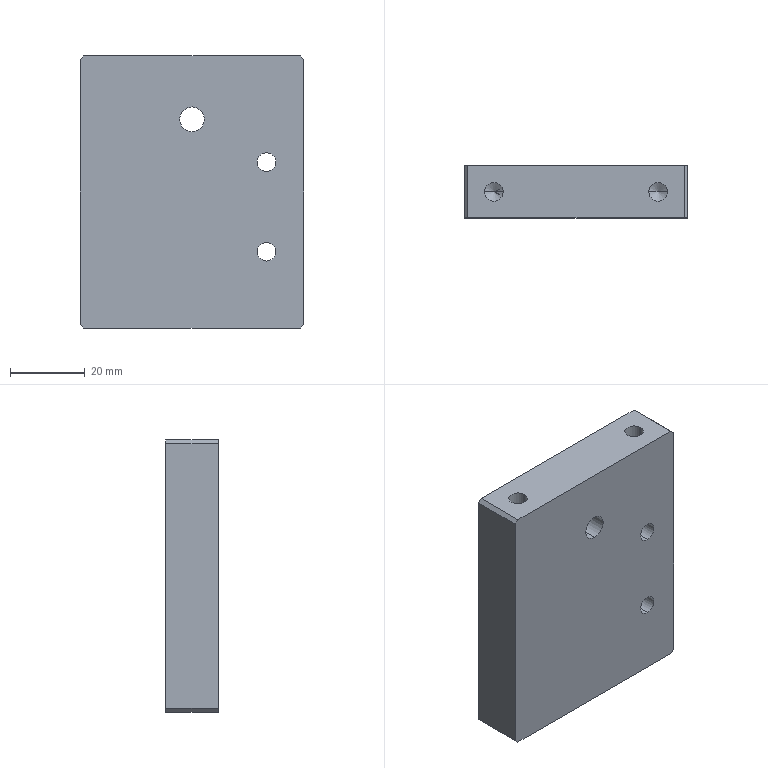Part | SolidWorks | features HoleWzd 3, Chamfer 1, Extrusion 1 | 1 solid | 27 faces | box 60 x 14 x 73 mm | volume 59241 mm3 | cylinder 12 | plane 11 | cone 4 | commonest cylinder face diameters 5 x8 6.6 x2 11 x2
STEP:
#1=CARTESIAN_POINT('',(0.,0.2,14.));
#2=VERTEX_POINT('',#1);
#3=CARTESIAN_POINT('',(0.,0.2,25.));
#4=VERTEX_POINT('',#3);
#5=CARTESIAN_POINT('',(0.,0.2,19.5));
#6=DIRECTION('',(0.,1.,0.));
#7=DIRECTION('',(0.,0.,1.));
#8=AXIS2_PLACEMENT_3D('',#5,#6,#7);
#9=CIRCLE('',#8,5.5);
#10=EDGE_CURVE('',#2,#4,#9,.T.);
#11=ORIENTED_EDGE('',*,*,#10,.F.);
#12=CARTESIAN_POINT('',(0.,7.,14.));
#13=VERTEX_POINT('',#12);
#14=CARTESIAN_POINT('',(0.,7.,14.));
#15=DIRECTION('',(0.,1.,0.));
#16=VECTOR('',#15,1000.);
#17=LINE('',#14,#16);
#18=EDGE_CURVE('',#2,#13,#17,.T.);
#19=ORIENTED_EDGE('',*,*,#18,.T.);
#20=CARTESIAN_POINT('',(0.,7.,25.));
#21=VERTEX_POINT('',#20);
#22=CARTESIAN_POINT('',(0.,7.,19.5));
#23=DIRECTION('',(0.,1.,0.));
#24=DIRECTION('',(0.,0.,1.));
#25=AXIS2_PLACEMENT_3D('',#22,#23,#24);
#26=CIRCLE('',#25,5.5);
#27=EDGE_CURVE('',#13,#21,#26,.T.);
#28=ORIENTED_EDGE('',*,*,#27,.T.);
#29=CARTESIAN_POINT('',(0.,7.,25.));
#30=DIRECTION('',(0.,1.,0.));
#31=VECTOR('',#30,1000.);
#32=LINE('',#29,#31);
#33=EDGE_CURVE('',#4,#21,#32,.T.);
#34=ORIENTED_EDGE('',*,*,#33,.F.);
#35=EDGE_LOOP('',(#11,#19,#28,#34));
#36=FACE_OUTER_BOUND('',#35,.T.);
#37=CARTESIAN_POINT('',(0.,7.,19.5));
#38=DIRECTION('',(0.,1.,0.));
#39=DIRECTION('',(0.,0.,1.));
#40=AXIS2_PLACEMENT_3D('',#37,#38,#39);
#41=CYLINDRICAL_SURFACE('',#40,5.5);
#42=ADVANCED_FACE('',(#36),#41,.F.);
#43=CARTESIAN_POINT('',(0.,-7.,16.2));
#44=VERTEX_POINT('',#43);
#45=CARTESIAN_POINT('',(0.,-7.,22.8));
#46=VERTEX_POINT('',#45);
#47=CARTESIAN_POINT('',(0.,-7.,19.5));
#48=DIRECTION('',(0.,1.,0.));
#49=DIRECTION('',(0.,0.,1.));
#50=AXIS2_PLACEMENT_3D('',#47,#48,#49);
#51=CIRCLE('',#50,3.3);
#52=EDGE_CURVE('',#44,#46,#51,.T.);
#53=ORIENTED_EDGE('',*,*,#52,.F.);
#54=CARTESIAN_POINT('',(0.,0.2,16.2));
#55=VERTEX_POINT('',#54);
#56=CARTESIAN_POINT('',(0.,7.,16.2));
#57=DIRECTION('',(0.,1.,0.));
#58=VECTOR('',#57,1000.);
#59=LINE('',#56,#58);
#60=EDGE_CURVE('',#44,#55,#59,.T.);
#61=ORIENTED_EDGE('',*,*,#60,.T.);
#62=CARTESIAN_POINT('',(0.,0.2,22.8));
#63=VERTEX_POINT('',#62);
#64=CARTESIAN_POINT('',(0.,0.2,19.5));
#65=DIRECTION('',(0.,1.,0.));
#66=DIRECTION('',(0.,0.,1.));
#67=AXIS2_PLACEMENT_3D('',#64,#65,#66);
#68=CIRCLE('',#67,3.3);
#69=EDGE_CURVE('',#55,#63,#68,.T.);
#70=ORIENTED_EDGE('',*,*,#69,.T.);
#71=CARTESIAN_POINT('',(0.,7.,22.8));
#72=DIRECTION('',(0.,1.,0.));
#73=VECTOR('',#72,1000.);
#74=LINE('',#71,#73);
#75=EDGE_CURVE('',#46,#63,#74,.T.);
#76=ORIENTED_EDGE('',*,*,#75,.F.);
#77=EDGE_LOOP('',(#53,#61,#70,#76));
#78=FACE_OUTER_BOUND('',#77,.T.);
#79=CARTESIAN_POINT('',(0.,7.,19.5));
#80=DIRECTION('',(0.,1.,0.));
#81=DIRECTION('',(0.,0.,1.));
#82=AXIS2_PLACEMENT_3D('',#79,#80,#81);
#83=CYLINDRICAL_SURFACE('',#82,3.3);
#84=ADVANCED_FACE('',(#78),#83,.F.);
#85=CARTESIAN_POINT('',(20.,-7.,-18.5));
#86=VERTEX_POINT('',#85);
#87=CARTESIAN_POINT('',(20.,-7.,-13.5));
#88=VERTEX_POINT('',#87);
#89=CARTESIAN_POINT('',(20.,-7.,-16.));
#90=DIRECTION('',(0.,1.,0.));
#91=DIRECTION('',(0.,0.,1.));
#92=AXIS2_PLACEMENT_3D('',#89,#90,#91);
#93=CIRCLE('',#92,2.5);
#94=EDGE_CURVE('',#86,#88,#93,.T.);
#95=ORIENTED_EDGE('',*,*,#94,.F.);
#96=CARTESIAN_POINT('',(20.,7.,-18.5));
#97=VERTEX_POINT('',#96);
#98=CARTESIAN_POINT('',(20.,7.,-18.5));
#99=DIRECTION('',(0.,1.,0.));
#100=VECTOR('',#99,1000.);
#101=LINE('',#98,#100);
#102=EDGE_CURVE('',#86,#97,#101,.T.);
#103=ORIENTED_EDGE('',*,*,#102,.T.);
#104=CARTESIAN_POINT('',(20.,7.,-13.5));
#105=VERTEX_POINT('',#104);
#106=CARTESIAN_POINT('',(20.,7.,-16.));
#107=DIRECTION('',(0.,1.,0.));
#108=DIRECTION('',(0.,0.,1.));
#109=AXIS2_PLACEMENT_3D('',#106,#107,#108);
#110=CIRCLE('',#109,2.5);
#111=EDGE_CURVE('',#97,#105,#110,.T.);
#112=ORIENTED_EDGE('',*,*,#111,.T.);
#113=CARTESIAN_POINT('',(20.,7.,-13.5));
#114=DIRECTION('',(0.,1.,0.));
#115=VECTOR('',#114,1000.);
#116=LINE('',#113,#115);
#117=EDGE_CURVE('',#88,#105,#116,.T.);
#118=ORIENTED_EDGE('',*,*,#117,.F.);
#119=EDGE_LOOP('',(#95,#103,#112,#118));
#120=FACE_OUTER_BOUND('',#119,.T.);
#121=CARTESIAN_POINT('',(20.,7.,-16.));
#122=DIRECTION('',(0.,1.,0.));
#123=DIRECTION('',(0.,0.,1.));
#124=AXIS2_PLACEMENT_3D('',#121,#122,#123);
#125=CYLINDRICAL_SURFACE('',#124,2.5);
#126=ADVANCED_FACE('',(#120),#125,.F.);
#127=CARTESIAN_POINT('',(20.,-7.,5.5));
#128=VERTEX_POINT('',#127);
#129=CARTESIAN_POINT('',(20.,-7.,10.5));
#130=VERTEX_POINT('',#129);
#131=CARTESIAN_POINT('',(20.,-7.,8.));
#132=DIRECTION('',(0.,1.,0.));
#133=DIRECTION('',(0.,0.,1.));
#134=AXIS2_PLACEMENT_3D('',#131,#132,#133);
#135=CIRCLE('',#134,2.5);
#136=EDGE_CURVE('',#128,#130,#135,.T.);
#137=ORIENTED_EDGE('',*,*,#136,.F.);
#138=CARTESIAN_POINT('',(20.,7.,5.5));
#139=VERTEX_POINT('',#138);
#140=CARTESIAN_POINT('',(20.,7.,5.5));
#141=DIRECTION('',(0.,1.,0.));
#142=VECTOR('',#141,1000.);
#143=LINE('',#140,#142);
#144=EDGE_CURVE('',#128,#139,#143,.T.);
#145=ORIENTED_EDGE('',*,*,#144,.T.);
#146=CARTESIAN_POINT('',(20.,7.,10.5));
#147=VERTEX_POINT('',#146);
#148=CARTESIAN_POINT('',(20.,7.,8.));
#149=DIRECTION('',(0.,1.,0.));
#150=DIRECTION('',(0.,0.,1.));
#151=AXIS2_PLACEMENT_3D('',#148,#149,#150);
#152=CIRCLE('',#151,2.5);
#153=EDGE_CURVE('',#139,#147,#152,.T.);
#154=ORIENTED_EDGE('',*,*,#153,.T.);
#155=CARTESIAN_POINT('',(20.,7.,10.5));
#156=DIRECTION('',(0.,1.,0.));
#157=VECTOR('',#156,1000.);
#158=LINE('',#155,#157);
#159=EDGE_CURVE('',#130,#147,#158,.T.);
#160=ORIENTED_EDGE('',*,*,#159,.F.);
#161=EDGE_LOOP('',(#137,#145,#154,#160));
#162=FACE_OUTER_BOUND('',#161,.T.);
#163=CARTESIAN_POINT('',(20.,7.,8.));
#164=DIRECTION('',(0.,1.,0.));
#165=DIRECTION('',(0.,0.,1.));
#166=AXIS2_PLACEMENT_3D('',#163,#164,#165);
#167=CYLINDRICAL_SURFACE('',#166,2.5);
#168=ADVANCED_FACE('',(#162),#167,.F.);
#169=CARTESIAN_POINT('',(-24.5,0.,21.5));
#170=VERTEX_POINT('',#169);
#171=CARTESIAN_POINT('',(-19.5,0.,21.5));
#172=VERTEX_POINT('',#171);
#173=CARTESIAN_POINT('',(-22.,0.,21.5));
#174=DIRECTION('',(0.,0.,1.));
#175=DIRECTION('',(1.,0.,0.));
#176=AXIS2_PLACEMENT_3D('',#173,#174,#175);
#177=CIRCLE('',#176,2.5);
#178=EDGE_CURVE('',#170,#172,#177,.T.);
#179=ORIENTED_EDGE('',*,*,#178,.F.);
#180=CARTESIAN_POINT('',(-24.5,0.,36.5));
#181=VERTEX_POINT('',#180);
#182=CARTESIAN_POINT('',(-24.5,0.,36.5));
#183=DIRECTION('',(0.,0.,1.));
#184=VECTOR('',#183,1000.);
#185=LINE('',#182,#184);
#186=EDGE_CURVE('',#170,#181,#185,.T.);
#187=ORIENTED_EDGE('',*,*,#186,.T.);
#188=CARTESIAN_POINT('',(-19.5,0.,36.5));
#189=VERTEX_POINT('',#188);
#190=CARTESIAN_POINT('',(-22.,0.,36.5));
#191=DIRECTION('',(0.,0.,1.));
#192=DIRECTION('',(1.,0.,0.));
#193=AXIS2_PLACEMENT_3D('',#190,#191,#192);
#194=CIRCLE('',#193,2.5);
#195=EDGE_CURVE('',#181,#189,#194,.T.);
#196=ORIENTED_EDGE('',*,*,#195,.T.);
#197=CARTESIAN_POINT('',(-19.5,0.,36.5));
#198=DIRECTION('',(0.,0.,1.));
#199=VECTOR('',#198,1000.);
#200=LINE('',#197,#199);
#201=EDGE_CURVE('',#172,#189,#200,.T.);
#202=ORIENTED_EDGE('',*,*,#201,.F.);
#203=EDGE_LOOP('',(#179,#187,#196,#202));
#204=FACE_OUTER_BOUND('',#203,.T.);
#205=CARTESIAN_POINT('',(-22.,0.,36.5));
#206=DIRECTION('',(0.,0.,1.));
#207=DIRECTION('',(1.,0.,0.));
#208=AXIS2_PLACEMENT_3D('',#205,#206,#207);
#209=CYLINDRICAL_SURFACE('',#208,2.5);
#210=ADVANCED_FACE('',(#204),#209,.F.);
#211=CARTESIAN_POINT('',(-22.,0.,19.998));
#212=VERTEX_POINT('',#211);
#213=CARTESIAN_POINT('',(-19.5,0.,21.5));
#214=DIRECTION('',(0.8572,0.,0.515));
#215=VECTOR('',#214,1000.);
#216=LINE('',#213,#215);
#217=EDGE_CURVE('',#212,#172,#216,.T.);
#218=ORIENTED_EDGE('',*,*,#217,.F.);
#219=CARTESIAN_POINT('',(-24.5,0.,21.5));
#220=DIRECTION('',(-0.8572,0.,0.515));
#221=VECTOR('',#220,1000.);
#222=LINE('',#219,#221);
#223=EDGE_CURVE('',#212,#170,#222,.T.);
#224=ORIENTED_EDGE('',*,*,#223,.T.);
#225=ORIENTED_EDGE('',*,*,#178,.T.);
#226=EDGE_LOOP('',(#218,#224,#225));
#227=FACE_OUTER_BOUND('',#226,.T.);
#228=CARTESIAN_POINT('',(-22.,0.,21.5));
#229=DIRECTION('',(0.,0.,1.));
#230=DIRECTION('',(1.,0.,0.));
#231=AXIS2_PLACEMENT_3D('',#228,#229,#230);
#232=CONICAL_SURFACE('',#231,2.5,1.03);
#233=ADVANCED_FACE('',(#227),#232,.F.);
#234=CARTESIAN_POINT('',(19.5,0.,21.5));
#235=VERTEX_POINT('',#234);
#236=CARTESIAN_POINT('',(24.5,0.,21.5));
#237=VERTEX_POINT('',#236);
#238=CARTESIAN_POINT('',(22.,0.,21.5));
#239=DIRECTION('',(0.,0.,1.));
#240=DIRECTION('',(1.,0.,0.));
#241=AXIS2_PLACEMENT_3D('',#238,#239,#240);
#242=CIRCLE('',#241,2.5);
#243=EDGE_CURVE('',#235,#237,#242,.T.);
#244=ORIENTED_EDGE('',*,*,#243,.F.);
#245=CARTESIAN_POINT('',(19.5,0.,36.5));
#246=VERTEX_POINT('',#245);
#247=CARTESIAN_POINT('',(19.5,0.,36.5));
#248=DIRECTION('',(0.,0.,1.));
#249=VECTOR('',#248,1000.);
#250=LINE('',#247,#249);
#251=EDGE_CURVE('',#235,#246,#250,.T.);
#252=ORIENTED_EDGE('',*,*,#251,.T.);
#253=CARTESIAN_POINT('',(24.5,0.,36.5));
#254=VERTEX_POINT('',#253);
#255=CARTESIAN_POINT('',(22.,0.,36.5));
#256=DIRECTION('',(0.,0.,1.));
#257=DIRECTION('',(1.,0.,0.));
#258=AXIS2_PLACEMENT_3D('',#255,#256,#257);
#259=CIRCLE('',#258,2.5);
#260=EDGE_CURVE('',#246,#254,#259,.T.);
#261=ORIENTED_EDGE('',*,*,#260,.T.);
#262=CARTESIAN_POINT('',(24.5,0.,36.5));
#263=DIRECTION('',(0.,0.,1.));
#264=VECTOR('',#263,1000.);
#265=LINE('',#262,#264);
#266=EDGE_CURVE('',#237,#254,#265,.T.);
#267=ORIENTED_EDGE('',*,*,#266,.F.);
#268=EDGE_LOOP('',(#244,#252,#261,#267));
#269=FACE_OUTER_BOUND('',#268,.T.);
#270=CARTESIAN_POINT('',(22.,0.,36.5));
#271=DIRECTION('',(0.,0.,1.));
#272=DIRECTION('',(1.,0.,0.));
#273=AXIS2_PLACEMENT_3D('',#270,#271,#272);
#274=CYLINDRICAL_SURFACE('',#273,2.5);
#275=ADVANCED_FACE('',(#269),#274,.F.);
#276=CARTESIAN_POINT('',(22.,0.,19.998));
#277=VERTEX_POINT('',#276);
#278=CARTESIAN_POINT('',(24.5,0.,21.5));
#279=DIRECTION('',(0.8572,0.,0.515));
#280=VECTOR('',#279,1000.);
#281=LINE('',#278,#280);
#282=EDGE_CURVE('',#277,#237,#281,.T.);
#283=ORIENTED_EDGE('',*,*,#282,.F.);
#284=CARTESIAN_POINT('',(19.5,0.,21.5));
#285=DIRECTION('',(-0.8572,0.,0.515));
#286=VECTOR('',#285,1000.);
#287=LINE('',#284,#286);
#288=EDGE_CURVE('',#277,#235,#287,.T.);
#289=ORIENTED_EDGE('',*,*,#288,.T.);
#290=ORIENTED_EDGE('',*,*,#243,.T.);
#291=EDGE_LOOP('',(#283,#289,#290));
#292=FACE_OUTER_BOUND('',#291,.T.);
#293=CARTESIAN_POINT('',(22.,0.,21.5));
#294=DIRECTION('',(0.,0.,1.));
#295=DIRECTION('',(1.,0.,0.));
#296=AXIS2_PLACEMENT_3D('',#293,#294,#295);
#297=CONICAL_SURFACE('',#296,2.5,1.03);
#298=ADVANCED_FACE('',(#292),#297,.F.);
#299=CARTESIAN_POINT('',(30.,-7.,35.5));
#300=VERTEX_POINT('',#299);
#301=CARTESIAN_POINT('',(30.,-7.,-35.5));
#302=VERTEX_POINT('',#301);
#303=CARTESIAN_POINT('',(30.,-7.,36.5));
#304=DIRECTION('',(0.,0.,-1.));
#305=VECTOR('',#304,1000.);
#306=LINE('',#303,#305);
#307=EDGE_CURVE('',#300,#302,#306,.T.);
#308=ORIENTED_EDGE('',*,*,#307,.T.);
#309=CARTESIAN_POINT('',(30.,7.,-35.5));
#310=VERTEX_POINT('',#309);
#311=CARTESIAN_POINT('',(30.,7.,-35.5));
#312=DIRECTION('',(0.,1.,0.));
#313=VECTOR('',#312,1000.);
#314=LINE('',#311,#313);
#315=EDGE_CURVE('',#302,#310,#314,.T.);
#316=ORIENTED_EDGE('',*,*,#315,.T.);
#317=CARTESIAN_POINT('',(30.,7.,35.5));
#318=VERTEX_POINT('',#317);
#319=CARTESIAN_POINT('',(30.,7.,36.5));
#320=DIRECTION('',(0.,0.,-1.));
#321=VECTOR('',#320,1000.);
#322=LINE('',#319,#321);
#323=EDGE_CURVE('',#318,#310,#322,.T.);
#324=ORIENTED_EDGE('',*,*,#323,.F.);
#325=CARTESIAN_POINT('',(30.,7.,35.5));
#326=DIRECTION('',(0.,-1.,0.));
#327=VECTOR('',#326,1000.);
#328=LINE('',#325,#327);
#329=EDGE_CURVE('',#318,#300,#328,.T.);
#330=ORIENTED_EDGE('',*,*,#329,.T.);
#331=EDGE_LOOP('',(#308,#316,#324,#330));
#332=FACE_OUTER_BOUND('',#331,.T.);
#333=CARTESIAN_POINT('',(30.,7.,36.5));
#334=DIRECTION('',(-1.,0.,0.));
#335=DIRECTION('',(0.,0.,1.));
#336=AXIS2_PLACEMENT_3D('',#333,#334,#335);
#337=PLANE('',#336);
#338=ADVANCED_FACE('',(#332),#337,.F.);
#339=CARTESIAN_POINT('',(29.,7.,-36.5));
#340=VERTEX_POINT('',#339);
#341=CARTESIAN_POINT('',(-29.,7.,-36.5));
#342=VERTEX_POINT('',#341);
#343=CARTESIAN_POINT('',(-30.,7.,-36.5));
#344=DIRECTION('',(-1.,0.,0.));
#345=VECTOR('',#344,1000.);
#346=LINE('',#343,#345);
#347=EDGE_CURVE('',#340,#342,#346,.T.);
#348=ORIENTED_EDGE('',*,*,#347,.F.);
#349=CARTESIAN_POINT('',(29.,-7.,-36.5));
#350=VERTEX_POINT('',#349);
#351=CARTESIAN_POINT('',(29.,7.,-36.5));
#352=DIRECTION('',(0.,-1.,0.));
#353=VECTOR('',#352,1000.);
#354=LINE('',#351,#353);
#355=EDGE_CURVE('',#340,#350,#354,.T.);
#356=ORIENTED_EDGE('',*,*,#355,.T.);
#357=CARTESIAN_POINT('',(-29.,-7.,-36.5));
#358=VERTEX_POINT('',#357);
#359=CARTESIAN_POINT('',(-30.,-7.,-36.5));
#360=DIRECTION('',(-1.,0.,0.));
#361=VECTOR('',#360,1000.);
#362=LINE('',#359,#361);
#363=EDGE_CURVE('',#350,#358,#362,.T.);
#364=ORIENTED_EDGE('',*,*,#363,.T.);
#365=CARTESIAN_POINT('',(-29.,7.,-36.5));
#366=DIRECTION('',(0.,1.,0.));
#367=VECTOR('',#366,1000.);
#368=LINE('',#365,#367);
#369=EDGE_CURVE('',#358,#342,#368,.T.);
#370=ORIENTED_EDGE('',*,*,#369,.T.);
#371=EDGE_LOOP('',(#348,#356,#364,#370));
#372=FACE_OUTER_BOUND('',#371,.T.);
#373=CARTESIAN_POINT('',(-30.,7.,-36.5));
#374=DIRECTION('',(0.,0.,1.));
#375=DIRECTION('',(1.,0.,0.));
#376=AXIS2_PLACEMENT_3D('',#373,#374,#375);
#377=PLANE('',#376);
#378=ADVANCED_FACE('',(#372),#377,.F.);
#379=CARTESIAN_POINT('',(-30.,7.,-35.5));
#380=VERTEX_POINT('',#379);
#381=CARTESIAN_POINT('',(-30.,7.,35.5));
#382=VERTEX_POINT('',#381);
#383=CARTESIAN_POINT('',(-30.,7.,36.5));
#384=DIRECTION('',(0.,0.,1.));
#385=VECTOR('',#384,1000.);
#386=LINE('',#383,#385);
#387=EDGE_CURVE('',#380,#382,#386,.T.);
#388=ORIENTED_EDGE('',*,*,#387,.F.);
#389=CARTESIAN_POINT('',(-30.,-7.,-35.5));
#390=VERTEX_POINT('',#389);
#391=CARTESIAN_POINT('',(-30.,7.,-35.5));
#392=DIRECTION('',(0.,-1.,0.));
#393=VECTOR('',#392,1000.);
#394=LINE('',#391,#393);
#395=EDGE_CURVE('',#380,#390,#394,.T.);
#396=ORIENTED_EDGE('',*,*,#395,.T.);
#397=CARTESIAN_POINT('',(-30.,-7.,35.5));
#398=VERTEX_POINT('',#397);
#399=CARTESIAN_POINT('',(-30.,-7.,36.5));
#400=DIRECTION('',(0.,0.,1.));
#401=VECTOR('',#400,1000.);
#402=LINE('',#399,#401);
#403=EDGE_CURVE('',#390,#398,#402,.T.);
#404=ORIENTED_EDGE('',*,*,#403,.T.);
#405=CARTESIAN_POINT('',(-30.,7.,35.5));
#406=DIRECTION('',(0.,1.,0.));
#407=VECTOR('',#406,1000.);
#408=LINE('',#405,#407);
#409=EDGE_CURVE('',#398,#382,#408,.T.);
#410=ORIENTED_EDGE('',*,*,#409,.T.);
#411=EDGE_LOOP('',(#388,#396,#404,#410));
#412=FACE_OUTER_BOUND('',#411,.T.);
#413=CARTESIAN_POINT('',(-30.,7.,36.5));
#414=DIRECTION('',(1.,0.,0.));
#415=DIRECTION('',(0.,0.,-1.));
#416=AXIS2_PLACEMENT_3D('',#413,#414,#415);
#417=PLANE('',#416);
#418=ADVANCED_FACE('',(#412),#417,.F.);
#419=CARTESIAN_POINT('',(-22.,0.,36.5));
#420=DIRECTION('',(0.,0.,1.));
#421=DIRECTION('',(1.,0.,0.));
#422=AXIS2_PLACEMENT_3D('',#419,#420,#421);
#423=CIRCLE('',#422,2.5);
#424=EDGE_CURVE('',#189,#181,#423,.T.);
#425=ORIENTED_EDGE('',*,*,#424,.F.);
#426=ORIENTED_EDGE('',*,*,#195,.F.);
#427=EDGE_LOOP('',(#425,#426));
#428=FACE_BOUND('',#427,.T.);
#429=CARTESIAN_POINT('',(22.,0.,36.5));
#430=DIRECTION('',(0.,0.,1.));
#431=DIRECTION('',(1.,0.,0.));
#432=AXIS2_PLACEMENT_3D('',#429,#430,#431);
#433=CIRCLE('',#432,2.5);
#434=EDGE_CURVE('',#254,#246,#433,.T.);
#435=ORIENTED_EDGE('',*,*,#434,.F.);
#436=ORIENTED_EDGE('',*,*,#260,.F.);
#437=EDGE_LOOP('',(#435,#436));
#438=FACE_BOUND('',#437,.T.);
#439=CARTESIAN_POINT('',(-29.,7.,36.5));
#440=VERTEX_POINT('',#439);
#441=CARTESIAN_POINT('',(29.,7.,36.5));
#442=VERTEX_POINT('',#441);
#443=CARTESIAN_POINT('',(-30.,7.,36.5));
#444=DIRECTION('',(1.,0.,0.));
#445=VECTOR('',#444,1000.);
#446=LINE('',#443,#445);
#447=EDGE_CURVE('',#440,#442,#446,.T.);
#448=ORIENTED_EDGE('',*,*,#447,.F.);
#449=CARTESIAN_POINT('',(-29.,-7.,36.5));
#450=VERTEX_POINT('',#449);
#451=CARTESIAN_POINT('',(-29.,7.,36.5));
#452=DIRECTION('',(0.,-1.,0.));
#453=VECTOR('',#452,1000.);
#454=LINE('',#451,#453);
#455=EDGE_CURVE('',#440,#450,#454,.T.);
#456=ORIENTED_EDGE('',*,*,#455,.T.);
#457=CARTESIAN_POINT('',(29.,-7.,36.5));
#458=VERTEX_POINT('',#457);
#459=CARTESIAN_POINT('',(-30.,-7.,36.5));
#460=DIRECTION('',(1.,0.,0.));
#461=VECTOR('',#460,1000.);
#462=LINE('',#459,#461);
#463=EDGE_CURVE('',#450,#458,#462,.T.);
#464=ORIENTED_EDGE('',*,*,#463,.T.);
#465=CARTESIAN_POINT('',(29.,7.,36.5));
#466=DIRECTION('',(0.,1.,0.));
#467=VECTOR('',#466,1000.);
#468=LINE('',#465,#467);
#469=EDGE_CURVE('',#458,#442,#468,.T.);
#470=ORIENTED_EDGE('',*,*,#469,.T.);
#471=EDGE_LOOP('',(#448,#456,#464,#470));
#472=FACE_OUTER_BOUND('',#471,.T.);
#473=CARTESIAN_POINT('',(-30.,7.,36.5));
#474=DIRECTION('',(0.,0.,-1.));
#475=DIRECTION('',(-1.,0.,0.));
#476=AXIS2_PLACEMENT_3D('',#473,#474,#475);
#477=PLANE('',#476);
#478=ADVANCED_FACE('',(#428,#438,#472),#477,.F.);
#479=CARTESIAN_POINT('',(0.,7.,19.5));
#480=DIRECTION('',(0.,1.,0.));
#481=DIRECTION('',(0.,0.,1.));
#482=AXIS2_PLACEMENT_3D('',#479,#480,#481);
#483=CIRCLE('',#482,5.5);
#484=EDGE_CURVE('',#21,#13,#483,.T.);
#485=ORIENTED_EDGE('',*,*,#484,.F.);
#486=ORIENTED_EDGE('',*,*,#27,.F.);
#487=EDGE_LOOP('',(#485,#486));
#488=FACE_BOUND('',#487,.T.);
#489=CARTESIAN_POINT('',(20.,7.,-16.));
#490=DIRECTION('',(0.,1.,0.));
#491=DIRECTION('',(0.,0.,1.));
#492=AXIS2_PLACEMENT_3D('',#489,#490,#491);
#493=CIRCLE('',#492,2.5);
#494=EDGE_CURVE('',#105,#97,#493,.T.);
#495=ORIENTED_EDGE('',*,*,#494,.F.);
#496=ORIENTED_EDGE('',*,*,#111,.F.);
#497=EDGE_LOOP('',(#495,#496));
#498=FACE_BOUND('',#497,.T.);
#499=CARTESIAN_POINT('',(20.,7.,8.));
#500=DIRECTION('',(0.,1.,0.));
#501=DIRECTION('',(0.,0.,1.));
#502=AXIS2_PLACEMENT_3D('',#499,#500,#501);
#503=CIRCLE('',#502,2.5);
#504=EDGE_CURVE('',#147,#139,#503,.T.);
#505=ORIENTED_EDGE('',*,*,#504,.F.);
#506=ORIENTED_EDGE('',*,*,#153,.F.);
#507=EDGE_LOOP('',(#505,#506));
#508=FACE_BOUND('',#507,.T.);
#509=ORIENTED_EDGE('',*,*,#323,.T.);
#510=CARTESIAN_POINT('',(29.,7.,-36.5));
#511=DIRECTION('',(-0.7071,0.,-0.7071));
#512=VECTOR('',#511,1000.);
#513=LINE('',#510,#512);
#514=EDGE_CURVE('',#310,#340,#513,.T.);
#515=ORIENTED_EDGE('',*,*,#514,.T.);
#516=ORIENTED_EDGE('',*,*,#347,.T.);
#517=CARTESIAN_POINT('',(-30.,7.,-35.5));
#518=DIRECTION('',(-0.7071,0.,0.7071));
#519=VECTOR('',#518,1000.);
#520=LINE('',#517,#519);
#521=EDGE_CURVE('',#342,#380,#520,.T.);
#522=ORIENTED_EDGE('',*,*,#521,.T.);
#523=ORIENTED_EDGE('',*,*,#387,.T.);
#524=CARTESIAN_POINT('',(-29.,7.,36.5));
#525=DIRECTION('',(0.7071,0.,0.7071));
#526=VECTOR('',#525,1000.);
#527=LINE('',#524,#526);
#528=EDGE_CURVE('',#382,#440,#527,.T.);
#529=ORIENTED_EDGE('',*,*,#528,.T.);
#530=ORIENTED_EDGE('',*,*,#447,.T.);
#531=CARTESIAN_POINT('',(30.,7.,35.5));
#532=DIRECTION('',(0.7071,0.,-0.7071));
#533=VECTOR('',#532,1000.);
#534=LINE('',#531,#533);
#535=EDGE_CURVE('',#442,#318,#534,.T.);
#536=ORIENTED_EDGE('',*,*,#535,.T.);
#537=EDGE_LOOP('',(#509,#515,#516,#522,#523,#529,#530,#536));
#538=FACE_OUTER_BOUND('',#537,.T.);
#539=CARTESIAN_POINT('',(0.,7.,0.));
#540=DIRECTION('',(0.,-1.,0.));
#541=DIRECTION('',(0.,0.,-1.));
#542=AXIS2_PLACEMENT_3D('',#539,#540,#541);
#543=PLANE('',#542);
#544=ADVANCED_FACE('',(#488,#498,#508,#538),#543,.F.);
#545=CARTESIAN_POINT('',(0.,-7.,19.5));
#546=DIRECTION('',(0.,1.,0.));
#547=DIRECTION('',(0.,0.,1.));
#548=AXIS2_PLACEMENT_3D('',#545,#546,#547);
#549=CIRCLE('',#548,3.3);
#550=EDGE_CURVE('',#46,#44,#549,.T.);
#551=ORIENTED_EDGE('',*,*,#550,.T.);
#552=ORIENTED_EDGE('',*,*,#52,.T.);
#553=EDGE_LOOP('',(#551,#552));
#554=FACE_BOUND('',#553,.T.);
#555=CARTESIAN_POINT('',(20.,-7.,-16.));
#556=DIRECTION('',(0.,1.,0.));
#557=DIRECTION('',(0.,0.,1.));
#558=AXIS2_PLACEMENT_3D('',#555,#556,#557);
#559=CIRCLE('',#558,2.5);
#560=EDGE_CURVE('',#88,#86,#559,.T.);
#561=ORIENTED_EDGE('',*,*,#560,.T.);
#562=ORIENTED_EDGE('',*,*,#94,.T.);
#563=EDGE_LOOP('',(#561,#562));
#564=FACE_BOUND('',#563,.T.);
#565=CARTESIAN_POINT('',(20.,-7.,8.));
#566=DIRECTION('',(0.,1.,0.));
#567=DIRECTION('',(0.,0.,1.));
#568=AXIS2_PLACEMENT_3D('',#565,#566,#567);
#569=CIRCLE('',#568,2.5);
#570=EDGE_CURVE('',#130,#128,#569,.T.);
#571=ORIENTED_EDGE('',*,*,#570,.T.);
#572=ORIENTED_EDGE('',*,*,#136,.T.);
#573=EDGE_LOOP('',(#571,#572));
#574=FACE_BOUND('',#573,.T.);
#575=ORIENTED_EDGE('',*,*,#363,.F.);
#576=CARTESIAN_POINT('',(32.75,-7.,-32.75));
#577=DIRECTION('',(0.7071,0.,0.7071));
#578=VECTOR('',#577,1000.);
#579=LINE('',#576,#578);
#580=EDGE_CURVE('',#350,#302,#579,.T.);
#581=ORIENTED_EDGE('',*,*,#580,.T.);
#582=ORIENTED_EDGE('',*,*,#307,.F.);
#583=CARTESIAN_POINT('',(32.75,-7.,32.75));
#584=DIRECTION('',(-0.7071,0.,0.7071));
#585=VECTOR('',#584,1000.);
#586=LINE('',#583,#585);
#587=EDGE_CURVE('',#300,#458,#586,.T.);
#588=ORIENTED_EDGE('',*,*,#587,.T.);
#589=ORIENTED_EDGE('',*,*,#463,.F.);
#590=CARTESIAN_POINT('',(-32.75,-7.,32.75));
#591=DIRECTION('',(-0.7071,0.,-0.7071));
#592=VECTOR('',#591,1000.);
#593=LINE('',#590,#592);
#594=EDGE_CURVE('',#450,#398,#593,.T.);
#595=ORIENTED_EDGE('',*,*,#594,.T.);
#596=ORIENTED_EDGE('',*,*,#403,.F.);
#597=CARTESIAN_POINT('',(-32.75,-7.,-32.75));
#598=DIRECTION('',(0.7071,0.,-0.7071));
#599=VECTOR('',#598,1000.);
#600=LINE('',#597,#599);
#601=EDGE_CURVE('',#390,#358,#600,.T.);
#602=ORIENTED_EDGE('',*,*,#601,.T.);
#603=EDGE_LOOP('',(#575,#581,#582,#588,#589,#595,#596,#602));
#604=FACE_OUTER_BOUND('',#603,.T.);
#605=CARTESIAN_POINT('',(0.,-7.,0.));
#606=DIRECTION('',(0.,-1.,0.));
#607=DIRECTION('',(0.,0.,-1.));
#608=AXIS2_PLACEMENT_3D('',#605,#606,#607);
#609=PLANE('',#608);
#610=ADVANCED_FACE('',(#554,#564,#574,#604),#609,.T.);
#611=ORIENTED_EDGE('',*,*,#288,.F.);
#612=ORIENTED_EDGE('',*,*,#282,.T.);
#613=CARTESIAN_POINT('',(22.,0.,21.5));
#614=DIRECTION('',(0.,0.,1.));
#615=DIRECTION('',(1.,0.,0.));
#616=AXIS2_PLACEMENT_3D('',#613,#614,#615);
#617=CIRCLE('',#616,2.5);
#618=EDGE_CURVE('',#237,#235,#617,.T.);
#619=ORIENTED_EDGE('',*,*,#618,.T.);
#620=EDGE_LOOP('',(#611,#612,#619));
#621=FACE_OUTER_BOUND('',#620,.T.);
#622=CARTESIAN_POINT('',(22.,0.,21.5));
#623=DIRECTION('',(0.,0.,1.));
#624=DIRECTION('',(1.,0.,0.));
#625=AXIS2_PLACEMENT_3D('',#622,#623,#624);
#626=CONICAL_SURFACE('',#625,2.5,1.03);
#627=ADVANCED_FACE('',(#621),#626,.F.);
#628=ORIENTED_EDGE('',*,*,#251,.F.);
#629=ORIENTED_EDGE('',*,*,#618,.F.);
#630=ORIENTED_EDGE('',*,*,#266,.T.);
#631=ORIENTED_EDGE('',*,*,#434,.T.);
#632=EDGE_LOOP('',(#628,#629,#630,#631));
#633=FACE_OUTER_BOUND('',#632,.T.);
#634=CARTESIAN_POINT('',(22.,0.,36.5));
#635=DIRECTION('',(0.,0.,1.));
#636=DIRECTION('',(1.,0.,0.));
#637=AXIS2_PLACEMENT_3D('',#634,#635,#636);
#638=CYLINDRICAL_SURFACE('',#637,2.5);
#639=ADVANCED_FACE('',(#633),#638,.F.);
#640=ORIENTED_EDGE('',*,*,#223,.F.);
#641=ORIENTED_EDGE('',*,*,#217,.T.);
#642=CARTESIAN_POINT('',(-22.,0.,21.5));
#643=DIRECTION('',(0.,0.,1.));
#644=DIRECTION('',(1.,0.,0.));
#645=AXIS2_PLACEMENT_3D('',#642,#643,#644);
#646=CIRCLE('',#645,2.5);
#647=EDGE_CURVE('',#172,#170,#646,.T.);
#648=ORIENTED_EDGE('',*,*,#647,.T.);
#649=EDGE_LOOP('',(#640,#641,#648));
#650=FACE_OUTER_BOUND('',#649,.T.);
#651=CARTESIAN_POINT('',(-22.,0.,21.5));
#652=DIRECTION('',(0.,0.,1.));
#653=DIRECTION('',(1.,0.,0.));
#654=AXIS2_PLACEMENT_3D('',#651,#652,#653);
#655=CONICAL_SURFACE('',#654,2.5,1.03);
#656=ADVANCED_FACE('',(#650),#655,.F.);
#657=ORIENTED_EDGE('',*,*,#186,.F.);
#658=ORIENTED_EDGE('',*,*,#647,.F.);
#659=ORIENTED_EDGE('',*,*,#201,.T.);
#660=ORIENTED_EDGE('',*,*,#424,.T.);
#661=EDGE_LOOP('',(#657,#658,#659,#660));
#662=FACE_OUTER_BOUND('',#661,.T.);
#663=CARTESIAN_POINT('',(-22.,0.,36.5));
#664=DIRECTION('',(0.,0.,1.));
#665=DIRECTION('',(1.,0.,0.));
#666=AXIS2_PLACEMENT_3D('',#663,#664,#665);
#667=CYLINDRICAL_SURFACE('',#666,2.5);
#668=ADVANCED_FACE('',(#662),#667,.F.);
#669=ORIENTED_EDGE('',*,*,#144,.F.);
#670=ORIENTED_EDGE('',*,*,#570,.F.);
#671=ORIENTED_EDGE('',*,*,#159,.T.);
#672=ORIENTED_EDGE('',*,*,#504,.T.);
#673=EDGE_LOOP('',(#669,#670,#671,#672));
#674=FACE_OUTER_BOUND('',#673,.T.);
#675=CARTESIAN_POINT('',(20.,7.,8.));
#676=DIRECTION('',(0.,1.,0.));
#677=DIRECTION('',(0.,0.,1.));
#678=AXIS2_PLACEMENT_3D('',#675,#676,#677);
#679=CYLINDRICAL_SURFACE('',#678,2.5);
#680=ADVANCED_FACE('',(#674),#679,.F.);
#681=ORIENTED_EDGE('',*,*,#102,.F.);
#682=ORIENTED_EDGE('',*,*,#560,.F.);
#683=ORIENTED_EDGE('',*,*,#117,.T.);
#684=ORIENTED_EDGE('',*,*,#494,.T.);
#685=EDGE_LOOP('',(#681,#682,#683,#684));
#686=FACE_OUTER_BOUND('',#685,.T.);
#687=CARTESIAN_POINT('',(20.,7.,-16.));
#688=DIRECTION('',(0.,1.,0.));
#689=DIRECTION('',(0.,0.,1.));
#690=AXIS2_PLACEMENT_3D('',#687,#688,#689);
#691=CYLINDRICAL_SURFACE('',#690,2.5);
#692=ADVANCED_FACE('',(#686),#691,.F.);
#693=ORIENTED_EDGE('',*,*,#514,.F.);
#694=ORIENTED_EDGE('',*,*,#315,.F.);
#695=ORIENTED_EDGE('',*,*,#580,.F.);
#696=ORIENTED_EDGE('',*,*,#355,.F.);
#697=EDGE_LOOP('',(#693,#694,#695,#696));
#698=FACE_OUTER_BOUND('',#697,.T.);
#699=CARTESIAN_POINT('',(29.,7.,-36.5));
#700=DIRECTION('',(-0.7071,0.,0.7071));
#701=DIRECTION('',(0.,-1.,0.));
#702=AXIS2_PLACEMENT_3D('',#699,#700,#701);
#703=PLANE('',#702);
#704=ADVANCED_FACE('',(#698),#703,.F.);
#705=ORIENTED_EDGE('',*,*,#521,.F.);
#706=ORIENTED_EDGE('',*,*,#369,.F.);
#707=ORIENTED_EDGE('',*,*,#601,.F.);
#708=ORIENTED_EDGE('',*,*,#395,.F.);
#709=EDGE_LOOP('',(#705,#706,#707,#708));
#710=FACE_OUTER_BOUND('',#709,.T.);
#711=CARTESIAN_POINT('',(-30.,7.,-35.5));
#712=DIRECTION('',(0.7071,0.,0.7071));
#713=DIRECTION('',(0.,-1.,0.));
#714=AXIS2_PLACEMENT_3D('',#711,#712,#713);
#715=PLANE('',#714);
#716=ADVANCED_FACE('',(#710),#715,.F.);
#717=ORIENTED_EDGE('',*,*,#528,.F.);
#718=ORIENTED_EDGE('',*,*,#409,.F.);
#719=ORIENTED_EDGE('',*,*,#594,.F.);
#720=ORIENTED_EDGE('',*,*,#455,.F.);
#721=EDGE_LOOP('',(#717,#718,#719,#720));
#722=FACE_OUTER_BOUND('',#721,.T.);
#723=CARTESIAN_POINT('',(-29.,7.,36.5));
#724=DIRECTION('',(0.7071,0.,-0.7071));
#725=DIRECTION('',(0.,-1.,0.));
#726=AXIS2_PLACEMENT_3D('',#723,#724,#725);
#727=PLANE('',#726);
#728=ADVANCED_FACE('',(#722),#727,.F.);
#729=ORIENTED_EDGE('',*,*,#535,.F.);
#730=ORIENTED_EDGE('',*,*,#469,.F.);
#731=ORIENTED_EDGE('',*,*,#587,.F.);
#732=ORIENTED_EDGE('',*,*,#329,.F.);
#733=EDGE_LOOP('',(#729,#730,#731,#732));
#734=FACE_OUTER_BOUND('',#733,.T.);
#735=CARTESIAN_POINT('',(30.,7.,35.5));
#736=DIRECTION('',(-0.7071,0.,-0.7071));
#737=DIRECTION('',(0.,-1.,0.));
#738=AXIS2_PLACEMENT_3D('',#735,#736,#737);
#739=PLANE('',#738);
#740=ADVANCED_FACE('',(#734),#739,.F.);
#741=ORIENTED_EDGE('',*,*,#60,.F.);
#742=ORIENTED_EDGE('',*,*,#550,.F.);
#743=ORIENTED_EDGE('',*,*,#75,.T.);
#744=CARTESIAN_POINT('',(0.,0.2,19.5));
#745=DIRECTION('',(0.,1.,0.));
#746=DIRECTION('',(0.,0.,1.));
#747=AXIS2_PLACEMENT_3D('',#744,#745,#746);
#748=CIRCLE('',#747,3.3);
#749=EDGE_CURVE('',#63,#55,#748,.T.);
#750=ORIENTED_EDGE('',*,*,#749,.T.);
#751=EDGE_LOOP('',(#741,#742,#743,#750));
#752=FACE_OUTER_BOUND('',#751,.T.);
#753=CARTESIAN_POINT('',(0.,7.,19.5));
#754=DIRECTION('',(0.,1.,0.));
#755=DIRECTION('',(0.,0.,1.));
#756=AXIS2_PLACEMENT_3D('',#753,#754,#755);
#757=CYLINDRICAL_SURFACE('',#756,3.3);
#758=ADVANCED_FACE('',(#752),#757,.F.);
#759=ORIENTED_EDGE('',*,*,#749,.F.);
#760=ORIENTED_EDGE('',*,*,#69,.F.);
#761=EDGE_LOOP('',(#759,#760));
#762=FACE_BOUND('',#761,.T.);
#763=CARTESIAN_POINT('',(0.,0.2,19.5));
#764=DIRECTION('',(0.,1.,0.));
#765=DIRECTION('',(0.,0.,1.));
#766=AXIS2_PLACEMENT_3D('',#763,#764,#765);
#767=CIRCLE('',#766,5.5);
#768=EDGE_CURVE('',#4,#2,#767,.T.);
#769=ORIENTED_EDGE('',*,*,#768,.T.);
#770=ORIENTED_EDGE('',*,*,#10,.T.);
#771=EDGE_LOOP('',(#769,#770));
#772=FACE_OUTER_BOUND('',#771,.T.);
#773=CARTESIAN_POINT('',(3.3,0.2,19.5));
#774=DIRECTION('',(0.,-1.,0.));
#775=DIRECTION('',(0.,0.,-1.));
#776=AXIS2_PLACEMENT_3D('',#773,#774,#775);
#777=PLANE('',#776);
#778=ADVANCED_FACE('',(#762,#772),#777,.F.);
#779=ORIENTED_EDGE('',*,*,#18,.F.);
#780=ORIENTED_EDGE('',*,*,#768,.F.);
#781=ORIENTED_EDGE('',*,*,#33,.T.);
#782=ORIENTED_EDGE('',*,*,#484,.T.);
#783=EDGE_LOOP('',(#779,#780,#781,#782));
#784=FACE_OUTER_BOUND('',#783,.T.);
#785=CARTESIAN_POINT('',(0.,7.,19.5));
#786=DIRECTION('',(0.,1.,0.));
#787=DIRECTION('',(0.,0.,1.));
#788=AXIS2_PLACEMENT_3D('',#785,#786,#787);
#789=CYLINDRICAL_SURFACE('',#788,5.5);
#790=ADVANCED_FACE('',(#784),#789,.F.);
#791=CLOSED_SHELL('',(#42,#84,#126,#168,#210,#233,#275,#298,#338,#378,#418,#478,#544,#610,#627,#639,#656,#668,#680,#692,#704,#716,#728,#740,#758,#778,#790));
#792=MANIFOLD_SOLID_BREP('',#791);
#793=CARTESIAN_POINT('',(0.,0.,0.));
#794=DIRECTION('',(0.,0.,1.));
#795=DIRECTION('',(1.,0.,0.));
#796=AXIS2_PLACEMENT_3D('',#793,#794,#795);
#797=(LENGTH_UNIT()NAMED_UNIT(*)SI_UNIT(.MILLI.,.METRE.));
#798=UNCERTAINTY_MEASURE_WITH_UNIT(LENGTH_MEASURE(0.00001),#797,'','');
#799=(NAMED_UNIT(*)PLANE_ANGLE_UNIT()SI_UNIT($,.RADIAN.));
#800=(NAMED_UNIT(*)SI_UNIT($,.STERADIAN.)SOLID_ANGLE_UNIT());
#801=(GEOMETRIC_REPRESENTATION_CONTEXT(3)GLOBAL_UNCERTAINTY_ASSIGNED_CONTEXT((#798))GLOBAL_UNIT_ASSIGNED_CONTEXT((#797,#799,#800))REPRESENTATION_CONTEXT('',''));
#802=ADVANCED_BREP_SHAPE_REPRESENTATION('',(#792,#796),#801);